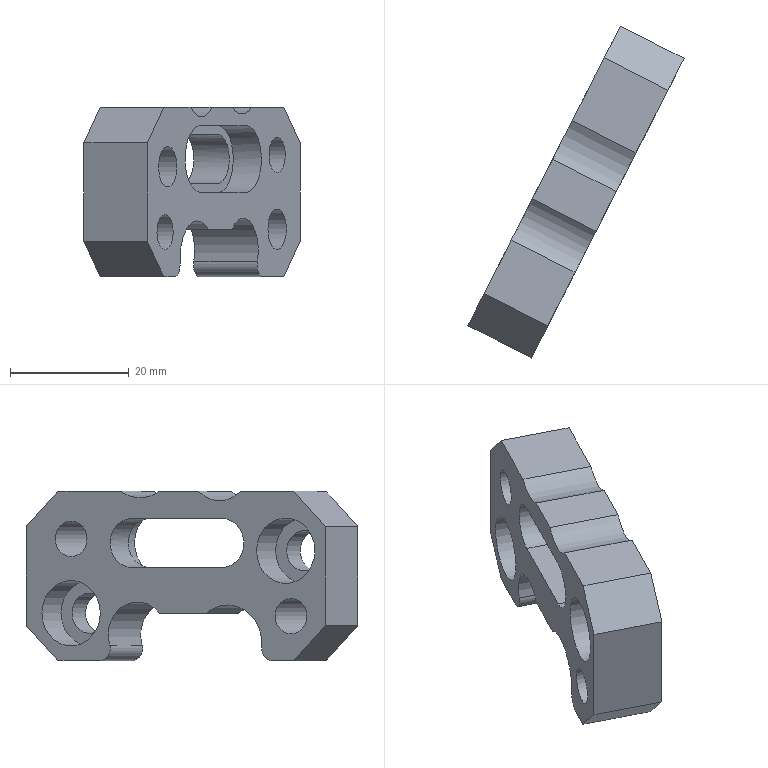Part | STEP file | gslz 2016.10.28-13_id78_x_t | 1 solid | 37 faces | box 36.343 x 55.79 x 28.5 mm | volume 10134 mm3 | plane 21 | cylinder 12 | spline 4 | commonest cylinder face diameters 11 x4 4 x2 6 x2 6.8 x2 13 x2